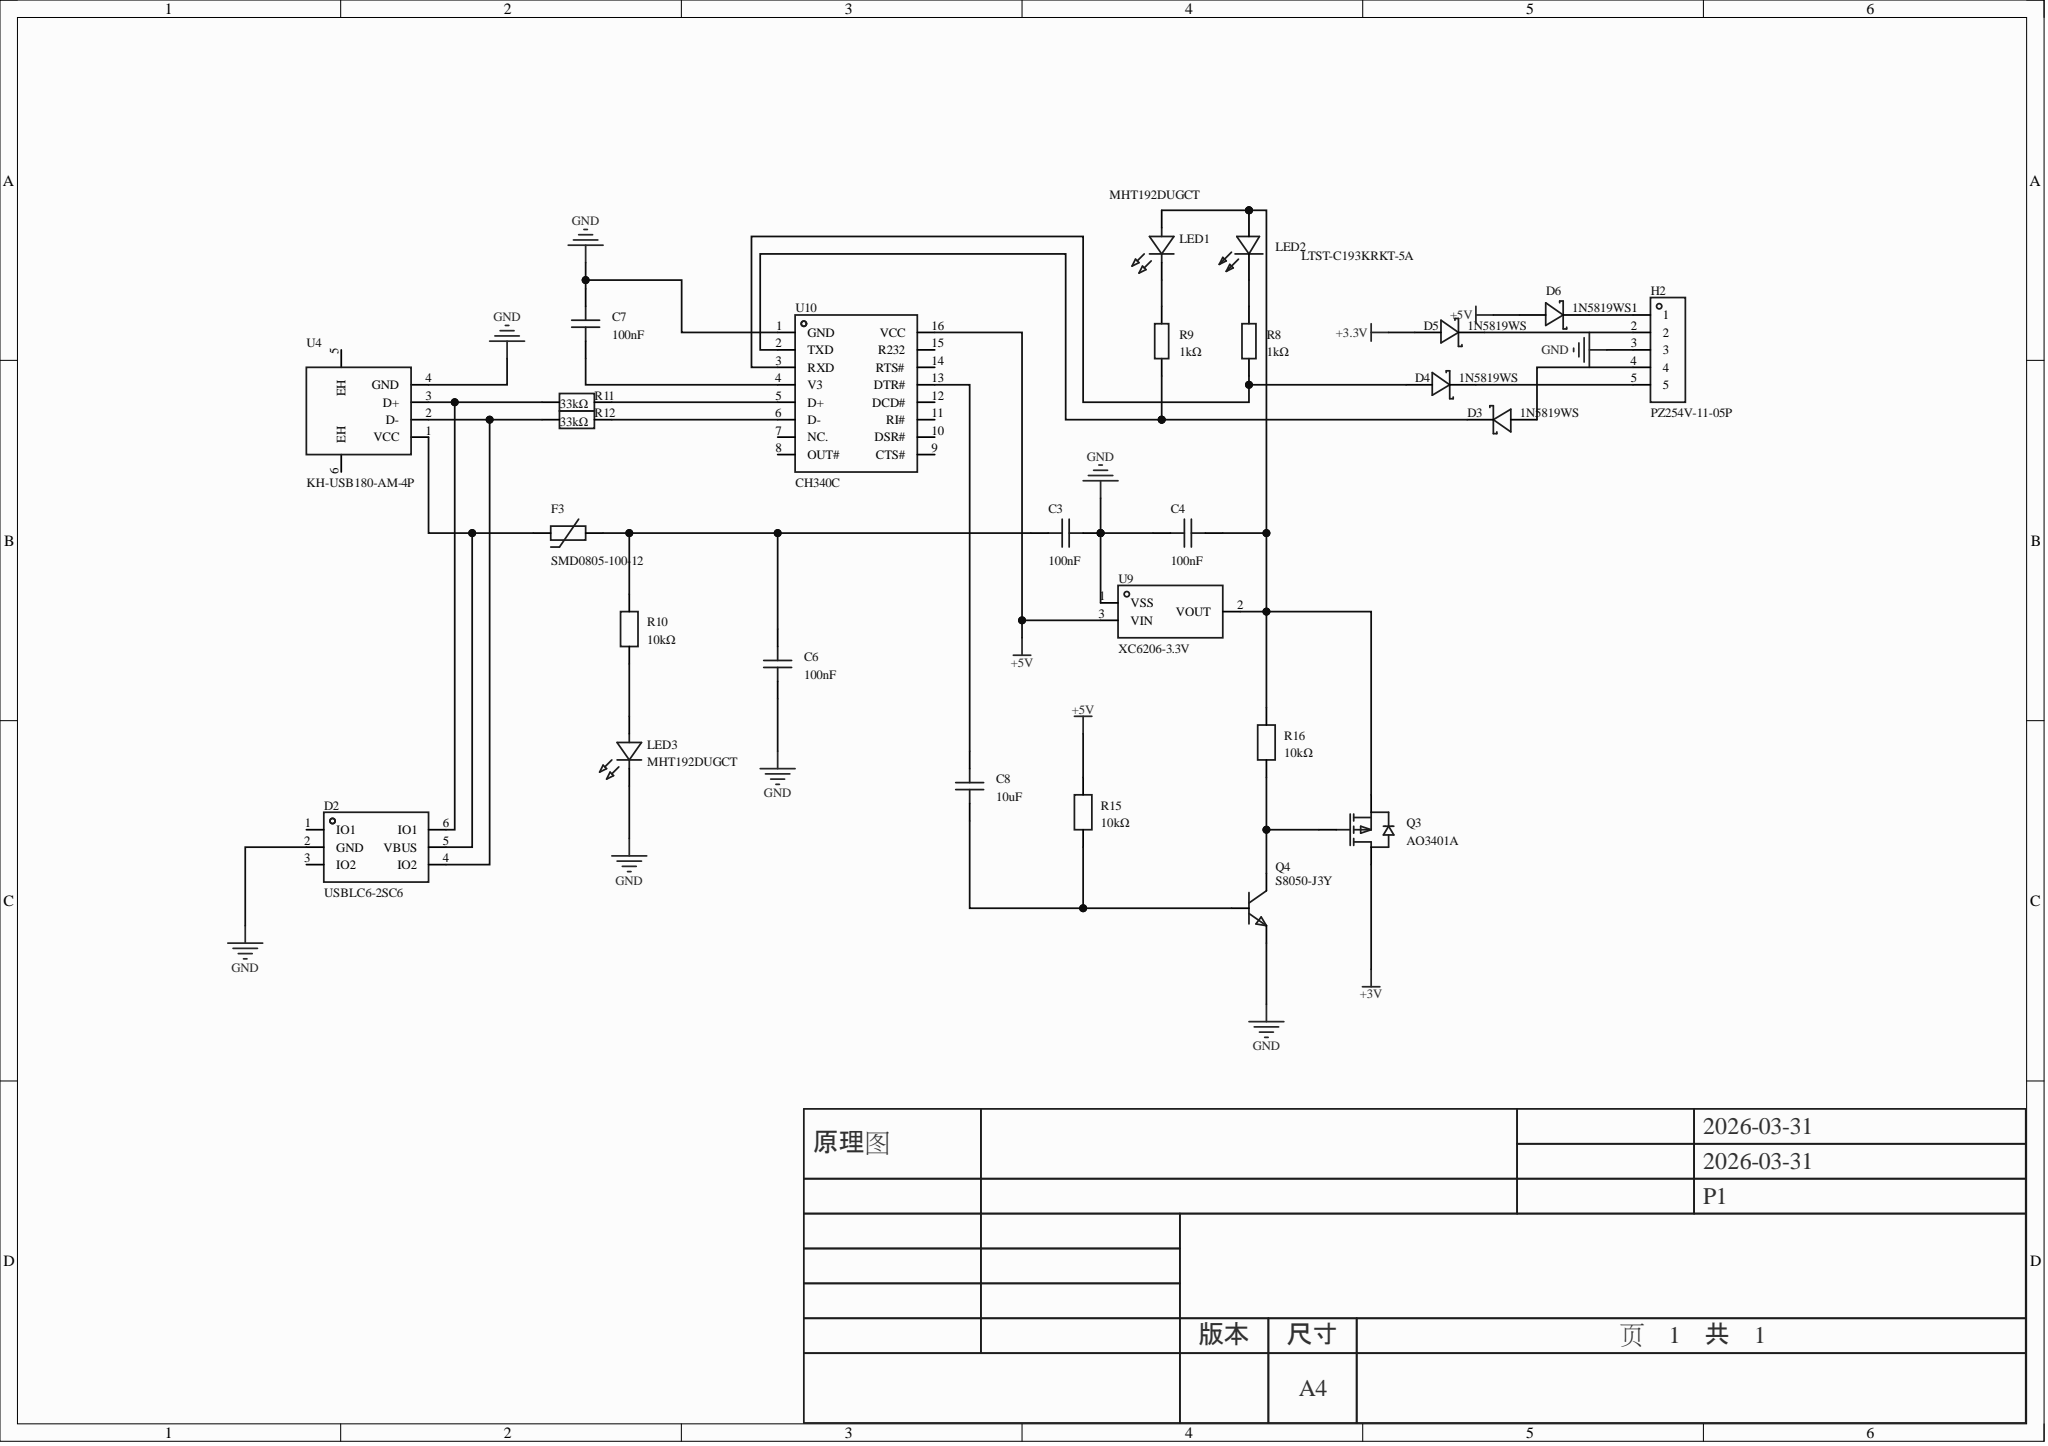Circuit board | Altium Designer | 27 parts | 22 nets
Bill of materials:
Comment,Description,Designator,Footprint,LibRef,Quantity
"100nF","","C3, C4, C6, C7","C0603","CGA0603X7R104K500JT, CC0603KRX7R9BB104","4"
"10uF","","C8","C0603","CL10A106MA8NRNC","1"
"USBLC6-2SC6","","D2","SOT-23-6_L2.9-W1.6-P0.95-LS2.8-BL","USBLC6-2SC6_C2827654","1"
"1N5819WS","","D3, D4, D5, D6","SOD-323_L1.8-W1.3-LS2.5-RD","1N5819WS_C191023","4"
"SMD0805-100-12","","F3","R0805","SMD0805-100-12","1"
"PZ254V-11-05P","","H2","HDR-TH_5P-P2.54-V-M","PZ254V-11-05P","1"
"MHT192DUGCT","","LED1, LED3","LED0603-RD","MHT192DUGCT","2"
"LTST-C193KRKT-5A","","LED2","LED0603-RD","LTST-C193KRKT-5A","1"
"AO3401A","","Q3","SOT-23_L2.9-W1.3-P1.90-LS2.4-BR","AO3401A_C15127","1"
"S8050-J3Y","","Q4","SOT-23-3_L2.9-W1.3-P0.95-LS2.4-BR-1","S8050-J3Y","1"
"1kΩ","","R8, R9","R0603","0603WAF1001T5E","2"
"10kΩ","","R10, R15, R16","R0603","FRC0603F1002TS","3"
"33kΩ","","R11, R12","R0603","FRC0603F3302TS","2"
"KH-USB180-AM-4P","","U4","USB-A-SMD_USB-A-1-TH","KH-USB180-AM-4P","1"
"XC6206-3.3V","","U9","SSOT-3_L2.9-W1.6-P0.95-LS2.8-BR","XC6206-3.3V","1"
"CH340C","","U10","SOP-16_L10.0-W3.9-P1.27-LS6.0-BL","CH340C","1"
Netlist (Protel format):
[
C3
C0603
100nF



]
[
C4
C0603
100nF



]
[
C6
C0603
100nF



]
[
C7
C0603
100nF



]
[
C8
C0603
10uF



]
[
D2
SOT-23-6_L2.9-W1.6-P0.95-LS2.8-BL
USBLC6-2SC6



]
[
D3
SOD-323_L1.8-W1.3-LS2.5-RD
1N5819WS



]
[
D4
SOD-323_L1.8-W1.3-LS2.5-RD
1N5819WS



]
[
D5
SOD-323_L1.8-W1.3-LS2.5-RD
1N5819WS



]
[
D6
SOD-323_L1.8-W1.3-LS2.5-RD
1N5819WS



]
[
F3
R0805
SMD0805-100-12



]
[
H2
HDR-TH_5P-P2.54-V-M
PZ254V-11-05P



]
[
LED1
LED0603-RD
MHT192DUGCT



]
[
LED2
LED0603-RD
LTST-C193KRKT-5A



]
[
LED3
LED0603-RD
MHT192DUGCT



]
[
Q3
SOT-23_L2.9-W1.3-P1.90-LS2.4-BR
AO3401A



]
[
Q4
SOT-23-3_L2.9-W1.3-P0.95-LS2.4-BR-1
S8050-J3Y



]
[
R8
R0603
1kΩ



]
[
R9
R0603
1kΩ



]
[
R10
R0603
10kΩ



]
[
R11
R0603
33kΩ



]
[
R12
R0603
33kΩ



]
[
R15
R0603
10kΩ



]
[
R16
R0603
10kΩ



]
[
U4
USB-A-SMD_USB-A-1-TH
KH-USB180-AM-4P



]
[
U9
SSOT-3_L2.9-W1.6-P0.95-LS2.8-BR
XC6206-3.3V



]
[
U10
SOP-16_L10.0-W3.9-P1.27-LS6.0-BL
CH340C



]
(
NetR12_2
R12-2
U10-6
)
(
NetR11_2
R11-2
U10-5
)
(
NetQ3_1
Q3-1
Q4-3
R16-1
)
(
NetLED3_2
LED3-2
R10-1
)
(
NetLED2_1
LED2-1
R8-2
)
(
NetLED1_1
LED1-1
R9-2
)
(
NetD6_1
D6-1
H2-1
)
(
NetD5_1
D5-1
H2-2
)
(
NetD4_2
D4-2
R8-1
U10-3
)
(
NetD4_1
D4-1
H2-5
)
(
NetD3_2
D3-2
H2-4
)
(
NetD3_1
D3-1
R9-1
U10-2
)
(
NetD2_6
D2-6
R11-1
U4-3
)
(
NetD2_5
D2-5
F3-1
U4-1
)
(
NetD2_4
D2-4
R12-1
U4-2
)
(
NetC8_2
C8-2
U10-13
)
(
NetC8_1
C8-1
Q4-1
R15-1
)
(
NetC7_1
C7-1
U10-4
)
(
NetC4_2
C4-2
LED1-2
LED2-2
Q3-2
R16-2
U9-2
)
(
NetC3_1
C3-1
C6-2
F3-2
R10-2
)
(
GND
C3-2
C4-1
C6-1
C7-2
D2-2
H2-3
LED3-1
Q4-2
U4-4
U9-1
U10-1
)
(
+5V
D6-2
R15-2
U9-3
U10-16
)